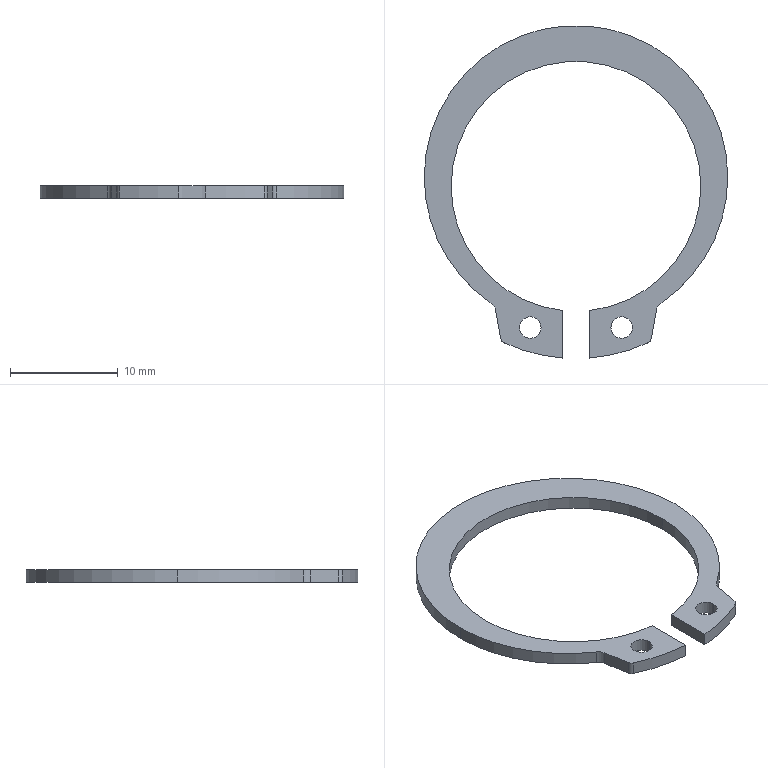Part | SolidWorks | features Extrusion 1 | 1 solid | 22 faces | box 28.2 x 30.881 x 1.2 mm | volume 270.422 mm3 | cylinder 16 | plane 6 | commonest cylinder face diameters 2 x6 23.2 x3 28.2 x3 1 x2 32 x2
STEP:
#1=CARTESIAN_POINT('',(-3.25,-13.959,0.));
#2=VERTEX_POINT('',#1);
#3=CARTESIAN_POINT('',(-5.25,-13.959,0.));
#4=VERTEX_POINT('',#3);
#5=CARTESIAN_POINT('',(-4.25,-13.959,0.));
#6=DIRECTION('',(0.,0.,-1.));
#7=DIRECTION('',(1.,0.,0.));
#8=AXIS2_PLACEMENT_3D('',#5,#6,#7);
#9=CIRCLE('',#8,1.);
#10=EDGE_CURVE('',#2,#4,#9,.T.);
#11=ORIENTED_EDGE('',*,*,#10,.F.);
#12=CARTESIAN_POINT('',(-3.25,-13.959,-1.2));
#13=VERTEX_POINT('',#12);
#14=CARTESIAN_POINT('',(-3.25,-13.959,0.));
#15=DIRECTION('',(0.,0.,-1.));
#16=VECTOR('',#15,1000.);
#17=LINE('',#14,#16);
#18=EDGE_CURVE('',#2,#13,#17,.T.);
#19=ORIENTED_EDGE('',*,*,#18,.T.);
#20=CARTESIAN_POINT('',(-5.25,-13.959,-1.2));
#21=VERTEX_POINT('',#20);
#22=CARTESIAN_POINT('',(-4.25,-13.959,-1.2));
#23=DIRECTION('',(0.,0.,-1.));
#24=DIRECTION('',(1.,0.,0.));
#25=AXIS2_PLACEMENT_3D('',#22,#23,#24);
#26=CIRCLE('',#25,1.);
#27=EDGE_CURVE('',#13,#21,#26,.T.);
#28=ORIENTED_EDGE('',*,*,#27,.T.);
#29=CARTESIAN_POINT('',(-5.25,-13.959,0.));
#30=DIRECTION('',(0.,0.,-1.));
#31=VECTOR('',#30,1000.);
#32=LINE('',#29,#31);
#33=EDGE_CURVE('',#4,#21,#32,.T.);
#34=ORIENTED_EDGE('',*,*,#33,.F.);
#35=EDGE_LOOP('',(#11,#19,#28,#34));
#36=FACE_OUTER_BOUND('',#35,.T.);
#37=CARTESIAN_POINT('',(-4.25,-13.959,0.));
#38=DIRECTION('',(0.,0.,-1.));
#39=DIRECTION('',(-1.,0.,0.));
#40=AXIS2_PLACEMENT_3D('',#37,#38,#39);
#41=CYLINDRICAL_SURFACE('',#40,1.);
#42=ADVANCED_FACE('',(#36),#41,.F.);
#43=CARTESIAN_POINT('',(5.25,-13.959,0.));
#44=VERTEX_POINT('',#43);
#45=CARTESIAN_POINT('',(3.25,-13.959,0.));
#46=VERTEX_POINT('',#45);
#47=CARTESIAN_POINT('',(4.25,-13.959,0.));
#48=DIRECTION('',(0.,0.,-1.));
#49=DIRECTION('',(1.,0.,0.));
#50=AXIS2_PLACEMENT_3D('',#47,#48,#49);
#51=CIRCLE('',#50,1.);
#52=EDGE_CURVE('',#44,#46,#51,.T.);
#53=ORIENTED_EDGE('',*,*,#52,.F.);
#54=CARTESIAN_POINT('',(5.25,-13.959,-1.2));
#55=VERTEX_POINT('',#54);
#56=CARTESIAN_POINT('',(5.25,-13.959,0.));
#57=DIRECTION('',(0.,0.,-1.));
#58=VECTOR('',#57,1000.);
#59=LINE('',#56,#58);
#60=EDGE_CURVE('',#44,#55,#59,.T.);
#61=ORIENTED_EDGE('',*,*,#60,.T.);
#62=CARTESIAN_POINT('',(3.25,-13.959,-1.2));
#63=VERTEX_POINT('',#62);
#64=CARTESIAN_POINT('',(4.25,-13.959,-1.2));
#65=DIRECTION('',(0.,0.,-1.));
#66=DIRECTION('',(1.,0.,0.));
#67=AXIS2_PLACEMENT_3D('',#64,#65,#66);
#68=CIRCLE('',#67,1.);
#69=EDGE_CURVE('',#55,#63,#68,.T.);
#70=ORIENTED_EDGE('',*,*,#69,.T.);
#71=CARTESIAN_POINT('',(3.25,-13.959,0.));
#72=DIRECTION('',(0.,0.,-1.));
#73=VECTOR('',#72,1000.);
#74=LINE('',#71,#73);
#75=EDGE_CURVE('',#46,#63,#74,.T.);
#76=ORIENTED_EDGE('',*,*,#75,.F.);
#77=EDGE_LOOP('',(#53,#61,#70,#76));
#78=FACE_OUTER_BOUND('',#77,.T.);
#79=CARTESIAN_POINT('',(4.25,-13.959,0.));
#80=DIRECTION('',(0.,0.,-1.));
#81=DIRECTION('',(-1.,0.,0.));
#82=AXIS2_PLACEMENT_3D('',#79,#80,#81);
#83=CYLINDRICAL_SURFACE('',#82,1.);
#84=ADVANCED_FACE('',(#78),#83,.F.);
#85=CARTESIAN_POINT('',(1.25,-12.362,0.));
#86=VERTEX_POINT('',#85);
#87=CARTESIAN_POINT('',(11.6,-0.83,0.));
#88=VERTEX_POINT('',#87);
#89=CARTESIAN_POINT('',(0.,-0.83,0.));
#90=DIRECTION('',(0.,0.,1.));
#91=DIRECTION('',(1.,0.,0.));
#92=AXIS2_PLACEMENT_3D('',#89,#90,#91);
#93=CIRCLE('',#92,11.6);
#94=EDGE_CURVE('',#86,#88,#93,.T.);
#95=ORIENTED_EDGE('',*,*,#94,.T.);
#96=CARTESIAN_POINT('',(11.6,-0.83,-1.2));
#97=VERTEX_POINT('',#96);
#98=CARTESIAN_POINT('',(11.6,-0.83,0.));
#99=DIRECTION('',(0.,0.,-1.));
#100=VECTOR('',#99,1000.);
#101=LINE('',#98,#100);
#102=EDGE_CURVE('',#88,#97,#101,.T.);
#103=ORIENTED_EDGE('',*,*,#102,.T.);
#104=CARTESIAN_POINT('',(1.25,-12.362,-1.2));
#105=VERTEX_POINT('',#104);
#106=CARTESIAN_POINT('',(0.,-0.83,-1.2));
#107=DIRECTION('',(0.,0.,1.));
#108=DIRECTION('',(1.,0.,0.));
#109=AXIS2_PLACEMENT_3D('',#106,#107,#108);
#110=CIRCLE('',#109,11.6);
#111=EDGE_CURVE('',#105,#97,#110,.T.);
#112=ORIENTED_EDGE('',*,*,#111,.F.);
#113=CARTESIAN_POINT('',(1.25,-12.362,0.));
#114=DIRECTION('',(0.,0.,-1.));
#115=VECTOR('',#114,1000.);
#116=LINE('',#113,#115);
#117=EDGE_CURVE('',#86,#105,#116,.T.);
#118=ORIENTED_EDGE('',*,*,#117,.F.);
#119=EDGE_LOOP('',(#95,#103,#112,#118));
#120=FACE_OUTER_BOUND('',#119,.T.);
#121=CARTESIAN_POINT('',(0.,-0.83,0.));
#122=DIRECTION('',(0.,0.,-1.));
#123=DIRECTION('',(-1.,0.,0.));
#124=AXIS2_PLACEMENT_3D('',#121,#122,#123);
#125=CYLINDRICAL_SURFACE('',#124,11.6);
#126=ADVANCED_FACE('',(#120),#125,.F.);
#127=ORIENTED_EDGE('',*,*,#102,.F.);
#128=CARTESIAN_POINT('',(-11.6,-0.83,0.));
#129=VERTEX_POINT('',#128);
#130=CARTESIAN_POINT('',(0.,-0.83,0.));
#131=DIRECTION('',(0.,0.,1.));
#132=DIRECTION('',(1.,0.,0.));
#133=AXIS2_PLACEMENT_3D('',#130,#131,#132);
#134=CIRCLE('',#133,11.6);
#135=EDGE_CURVE('',#88,#129,#134,.T.);
#136=ORIENTED_EDGE('',*,*,#135,.T.);
#137=CARTESIAN_POINT('',(-11.6,-0.83,-1.2));
#138=VERTEX_POINT('',#137);
#139=CARTESIAN_POINT('',(-11.6,-0.83,0.));
#140=DIRECTION('',(0.,0.,-1.));
#141=VECTOR('',#140,1000.);
#142=LINE('',#139,#141);
#143=EDGE_CURVE('',#129,#138,#142,.T.);
#144=ORIENTED_EDGE('',*,*,#143,.T.);
#145=CARTESIAN_POINT('',(0.,-0.83,-1.2));
#146=DIRECTION('',(0.,0.,1.));
#147=DIRECTION('',(1.,0.,0.));
#148=AXIS2_PLACEMENT_3D('',#145,#146,#147);
#149=CIRCLE('',#148,11.6);
#150=EDGE_CURVE('',#97,#138,#149,.T.);
#151=ORIENTED_EDGE('',*,*,#150,.F.);
#152=EDGE_LOOP('',(#127,#136,#144,#151));
#153=FACE_OUTER_BOUND('',#152,.T.);
#154=CARTESIAN_POINT('',(0.,-0.83,0.));
#155=DIRECTION('',(0.,0.,-1.));
#156=DIRECTION('',(-1.,0.,0.));
#157=AXIS2_PLACEMENT_3D('',#154,#155,#156);
#158=CYLINDRICAL_SURFACE('',#157,11.6);
#159=ADVANCED_FACE('',(#153),#158,.F.);
#160=CARTESIAN_POINT('',(-14.1,0.,0.));
#161=VERTEX_POINT('',#160);
#162=CARTESIAN_POINT('',(14.1,0.,0.));
#163=VERTEX_POINT('',#162);
#164=CARTESIAN_POINT('',(0.,0.,0.));
#165=DIRECTION('',(0.,0.,-1.));
#166=DIRECTION('',(-1.,0.,0.));
#167=AXIS2_PLACEMENT_3D('',#164,#165,#166);
#168=CIRCLE('',#167,14.1);
#169=EDGE_CURVE('',#161,#163,#168,.T.);
#170=ORIENTED_EDGE('',*,*,#169,.T.);
#171=CARTESIAN_POINT('',(14.1,0.,-1.2));
#172=VERTEX_POINT('',#171);
#173=CARTESIAN_POINT('',(14.1,0.,0.));
#174=DIRECTION('',(0.,0.,-1.));
#175=VECTOR('',#174,1000.);
#176=LINE('',#173,#175);
#177=EDGE_CURVE('',#163,#172,#176,.T.);
#178=ORIENTED_EDGE('',*,*,#177,.T.);
#179=CARTESIAN_POINT('',(-14.1,0.,-1.2));
#180=VERTEX_POINT('',#179);
#181=CARTESIAN_POINT('',(0.,0.,-1.2));
#182=DIRECTION('',(0.,0.,-1.));
#183=DIRECTION('',(-1.,0.,0.));
#184=AXIS2_PLACEMENT_3D('',#181,#182,#183);
#185=CIRCLE('',#184,14.1);
#186=EDGE_CURVE('',#180,#172,#185,.T.);
#187=ORIENTED_EDGE('',*,*,#186,.F.);
#188=CARTESIAN_POINT('',(-14.1,0.,0.));
#189=DIRECTION('',(0.,0.,-1.));
#190=VECTOR('',#189,1000.);
#191=LINE('',#188,#190);
#192=EDGE_CURVE('',#161,#180,#191,.T.);
#193=ORIENTED_EDGE('',*,*,#192,.F.);
#194=EDGE_LOOP('',(#170,#178,#187,#193));
#195=FACE_OUTER_BOUND('',#194,.T.);
#196=CARTESIAN_POINT('',(0.,0.,0.));
#197=DIRECTION('',(0.,0.,-1.));
#198=DIRECTION('',(-1.,0.,0.));
#199=AXIS2_PLACEMENT_3D('',#196,#197,#198);
#200=CYLINDRICAL_SURFACE('',#199,14.1);
#201=ADVANCED_FACE('',(#195),#200,.T.);
#202=CARTESIAN_POINT('',(-7.893,-11.684,0.));
#203=VERTEX_POINT('',#202);
#204=CARTESIAN_POINT('',(0.,0.,0.));
#205=DIRECTION('',(0.,0.,-1.));
#206=DIRECTION('',(-1.,0.,0.));
#207=AXIS2_PLACEMENT_3D('',#204,#205,#206);
#208=CIRCLE('',#207,14.1);
#209=EDGE_CURVE('',#203,#161,#208,.T.);
#210=ORIENTED_EDGE('',*,*,#209,.T.);
#211=ORIENTED_EDGE('',*,*,#192,.T.);
#212=CARTESIAN_POINT('',(-7.893,-11.684,-1.2));
#213=VERTEX_POINT('',#212);
#214=CARTESIAN_POINT('',(0.,0.,-1.2));
#215=DIRECTION('',(0.,0.,-1.));
#216=DIRECTION('',(-1.,0.,0.));
#217=AXIS2_PLACEMENT_3D('',#214,#215,#216);
#218=CIRCLE('',#217,14.1);
#219=EDGE_CURVE('',#213,#180,#218,.T.);
#220=ORIENTED_EDGE('',*,*,#219,.F.);
#221=CARTESIAN_POINT('',(-7.893,-11.684,0.));
#222=DIRECTION('',(0.,0.,-1.));
#223=VECTOR('',#222,1000.);
#224=LINE('',#221,#223);
#225=EDGE_CURVE('',#203,#213,#224,.T.);
#226=ORIENTED_EDGE('',*,*,#225,.F.);
#227=EDGE_LOOP('',(#210,#211,#220,#226));
#228=FACE_OUTER_BOUND('',#227,.T.);
#229=CARTESIAN_POINT('',(0.,0.,0.));
#230=DIRECTION('',(0.,0.,-1.));
#231=DIRECTION('',(-1.,0.,0.));
#232=AXIS2_PLACEMENT_3D('',#229,#230,#231);
#233=CYLINDRICAL_SURFACE('',#232,14.1);
#234=ADVANCED_FACE('',(#228),#233,.T.);
#235=CARTESIAN_POINT('',(6.719,-15.351,-1.2));
#236=VERTEX_POINT('',#235);
#237=CARTESIAN_POINT('',(1.25,-16.781,-1.2));
#238=VERTEX_POINT('',#237);
#239=CARTESIAN_POINT('',(0.,-0.83,-1.2));
#240=DIRECTION('',(0.,0.,-1.));
#241=DIRECTION('',(-1.,0.,0.));
#242=AXIS2_PLACEMENT_3D('',#239,#240,#241);
#243=CIRCLE('',#242,16.);
#244=EDGE_CURVE('',#236,#238,#243,.T.);
#245=ORIENTED_EDGE('',*,*,#244,.F.);
#246=CARTESIAN_POINT('',(6.719,-15.351,0.));
#247=VERTEX_POINT('',#246);
#248=CARTESIAN_POINT('',(6.719,-15.351,0.));
#249=DIRECTION('',(0.,0.,-1.));
#250=VECTOR('',#249,1000.);
#251=LINE('',#248,#250);
#252=EDGE_CURVE('',#247,#236,#251,.T.);
#253=ORIENTED_EDGE('',*,*,#252,.F.);
#254=CARTESIAN_POINT('',(1.25,-16.781,0.));
#255=VERTEX_POINT('',#254);
#256=CARTESIAN_POINT('',(0.,-0.83,0.));
#257=DIRECTION('',(0.,0.,-1.));
#258=DIRECTION('',(-1.,0.,0.));
#259=AXIS2_PLACEMENT_3D('',#256,#257,#258);
#260=CIRCLE('',#259,16.);
#261=EDGE_CURVE('',#247,#255,#260,.T.);
#262=ORIENTED_EDGE('',*,*,#261,.T.);
#263=CARTESIAN_POINT('',(1.25,-16.781,0.));
#264=DIRECTION('',(0.,0.,-1.));
#265=VECTOR('',#264,1000.);
#266=LINE('',#263,#265);
#267=EDGE_CURVE('',#255,#238,#266,.T.);
#268=ORIENTED_EDGE('',*,*,#267,.T.);
#269=EDGE_LOOP('',(#245,#253,#262,#268));
#270=FACE_OUTER_BOUND('',#269,.T.);
#271=CARTESIAN_POINT('',(0.,-0.83,0.));
#272=DIRECTION('',(0.,0.,-1.));
#273=DIRECTION('',(-1.,0.,0.));
#274=AXIS2_PLACEMENT_3D('',#271,#272,#273);
#275=CYLINDRICAL_SURFACE('',#274,16.);
#276=ADVANCED_FACE('',(#270),#275,.T.);
#277=CARTESIAN_POINT('',(7.002,-14.984,-1.2));
#278=VERTEX_POINT('',#277);
#279=CARTESIAN_POINT('',(6.509,-14.897,-1.2));
#280=DIRECTION('',(0.,0.,-1.));
#281=DIRECTION('',(-1.,0.,0.));
#282=AXIS2_PLACEMENT_3D('',#279,#280,#281);
#283=CIRCLE('',#282,0.5);
#284=EDGE_CURVE('',#278,#236,#283,.T.);
#285=ORIENTED_EDGE('',*,*,#284,.F.);
#286=CARTESIAN_POINT('',(7.002,-14.984,0.));
#287=VERTEX_POINT('',#286);
#288=CARTESIAN_POINT('',(7.002,-14.984,0.));
#289=DIRECTION('',(0.,0.,-1.));
#290=VECTOR('',#289,1000.);
#291=LINE('',#288,#290);
#292=EDGE_CURVE('',#287,#278,#291,.T.);
#293=ORIENTED_EDGE('',*,*,#292,.F.);
#294=CARTESIAN_POINT('',(6.509,-14.897,0.));
#295=DIRECTION('',(0.,0.,-1.));
#296=DIRECTION('',(-1.,0.,0.));
#297=AXIS2_PLACEMENT_3D('',#294,#295,#296);
#298=CIRCLE('',#297,0.5);
#299=EDGE_CURVE('',#287,#247,#298,.T.);
#300=ORIENTED_EDGE('',*,*,#299,.T.);
#301=ORIENTED_EDGE('',*,*,#252,.T.);
#302=EDGE_LOOP('',(#285,#293,#300,#301));
#303=FACE_OUTER_BOUND('',#302,.T.);
#304=CARTESIAN_POINT('',(6.509,-14.897,0.));
#305=DIRECTION('',(0.,0.,-1.));
#306=DIRECTION('',(-1.,0.,0.));
#307=AXIS2_PLACEMENT_3D('',#304,#305,#306);
#308=CYLINDRICAL_SURFACE('',#307,0.5);
#309=ADVANCED_FACE('',(#303),#308,.T.);
#310=CARTESIAN_POINT('',(7.468,-12.339,-1.2));
#311=VERTEX_POINT('',#310);
#312=CARTESIAN_POINT('',(7.468,-12.339,-1.2));
#313=DIRECTION('',(-0.1736,-0.9848,0.));
#314=VECTOR('',#313,1000.);
#315=LINE('',#312,#314);
#316=EDGE_CURVE('',#311,#278,#315,.T.);
#317=ORIENTED_EDGE('',*,*,#316,.F.);
#318=CARTESIAN_POINT('',(7.468,-12.339,0.));
#319=VERTEX_POINT('',#318);
#320=CARTESIAN_POINT('',(7.468,-12.339,0.));
#321=DIRECTION('',(0.,0.,-1.));
#322=VECTOR('',#321,1000.);
#323=LINE('',#320,#322);
#324=EDGE_CURVE('',#319,#311,#323,.T.);
#325=ORIENTED_EDGE('',*,*,#324,.F.);
#326=CARTESIAN_POINT('',(7.468,-12.339,0.));
#327=DIRECTION('',(-0.1736,-0.9848,0.));
#328=VECTOR('',#327,1000.);
#329=LINE('',#326,#328);
#330=EDGE_CURVE('',#319,#287,#329,.T.);
#331=ORIENTED_EDGE('',*,*,#330,.T.);
#332=ORIENTED_EDGE('',*,*,#292,.T.);
#333=EDGE_LOOP('',(#317,#325,#331,#332));
#334=FACE_OUTER_BOUND('',#333,.T.);
#335=CARTESIAN_POINT('',(7.468,-12.339,0.));
#336=DIRECTION('',(0.9848,-0.1736,0.));
#337=DIRECTION('',(0.1736,0.9848,0.));
#338=AXIS2_PLACEMENT_3D('',#335,#336,#337);
#339=PLANE('',#338);
#340=ADVANCED_FACE('',(#334),#339,.T.);
#341=CARTESIAN_POINT('',(7.893,-11.684,-1.2));
#342=VERTEX_POINT('',#341);
#343=CARTESIAN_POINT('',(8.453,-12.512,-1.2));
#344=DIRECTION('',(0.,0.,1.));
#345=DIRECTION('',(1.,0.,0.));
#346=AXIS2_PLACEMENT_3D('',#343,#344,#345);
#347=CIRCLE('',#346,1.);
#348=EDGE_CURVE('',#342,#311,#347,.T.);
#349=ORIENTED_EDGE('',*,*,#348,.F.);
#350=CARTESIAN_POINT('',(7.893,-11.684,0.));
#351=VERTEX_POINT('',#350);
#352=CARTESIAN_POINT('',(7.893,-11.684,0.));
#353=DIRECTION('',(0.,0.,-1.));
#354=VECTOR('',#353,1000.);
#355=LINE('',#352,#354);
#356=EDGE_CURVE('',#351,#342,#355,.T.);
#357=ORIENTED_EDGE('',*,*,#356,.F.);
#358=CARTESIAN_POINT('',(8.453,-12.512,0.));
#359=DIRECTION('',(0.,0.,1.));
#360=DIRECTION('',(1.,0.,0.));
#361=AXIS2_PLACEMENT_3D('',#358,#359,#360);
#362=CIRCLE('',#361,1.);
#363=EDGE_CURVE('',#351,#319,#362,.T.);
#364=ORIENTED_EDGE('',*,*,#363,.T.);
#365=ORIENTED_EDGE('',*,*,#324,.T.);
#366=EDGE_LOOP('',(#349,#357,#364,#365));
#367=FACE_OUTER_BOUND('',#366,.T.);
#368=CARTESIAN_POINT('',(8.453,-12.512,0.));
#369=DIRECTION('',(0.,0.,-1.));
#370=DIRECTION('',(-1.,0.,0.));
#371=AXIS2_PLACEMENT_3D('',#368,#369,#370);
#372=CYLINDRICAL_SURFACE('',#371,1.);
#373=ADVANCED_FACE('',(#367),#372,.F.);
#374=ORIENTED_EDGE('',*,*,#177,.F.);
#375=CARTESIAN_POINT('',(0.,0.,0.));
#376=DIRECTION('',(0.,0.,-1.));
#377=DIRECTION('',(-1.,0.,0.));
#378=AXIS2_PLACEMENT_3D('',#375,#376,#377);
#379=CIRCLE('',#378,14.1);
#380=EDGE_CURVE('',#163,#351,#379,.T.);
#381=ORIENTED_EDGE('',*,*,#380,.T.);
#382=ORIENTED_EDGE('',*,*,#356,.T.);
#383=CARTESIAN_POINT('',(0.,0.,-1.2));
#384=DIRECTION('',(0.,0.,-1.));
#385=DIRECTION('',(-1.,0.,0.));
#386=AXIS2_PLACEMENT_3D('',#383,#384,#385);
#387=CIRCLE('',#386,14.1);
#388=EDGE_CURVE('',#172,#342,#387,.T.);
#389=ORIENTED_EDGE('',*,*,#388,.F.);
#390=EDGE_LOOP('',(#374,#381,#382,#389));
#391=FACE_OUTER_BOUND('',#390,.T.);
#392=CARTESIAN_POINT('',(0.,0.,0.));
#393=DIRECTION('',(0.,0.,-1.));
#394=DIRECTION('',(-1.,0.,0.));
#395=AXIS2_PLACEMENT_3D('',#392,#393,#394);
#396=CYLINDRICAL_SURFACE('',#395,14.1);
#397=ADVANCED_FACE('',(#391),#396,.T.);
#398=CARTESIAN_POINT('',(-7.468,-12.339,-1.2));
#399=VERTEX_POINT('',#398);
#400=CARTESIAN_POINT('',(-8.453,-12.512,-1.2));
#401=DIRECTION('',(0.,0.,1.));
#402=DIRECTION('',(1.,0.,0.));
#403=AXIS2_PLACEMENT_3D('',#400,#401,#402);
#404=CIRCLE('',#403,1.);
#405=EDGE_CURVE('',#399,#213,#404,.T.);
#406=ORIENTED_EDGE('',*,*,#405,.F.);
#407=CARTESIAN_POINT('',(-7.468,-12.339,0.));
#408=VERTEX_POINT('',#407);
#409=CARTESIAN_POINT('',(-7.468,-12.339,0.));
#410=DIRECTION('',(0.,0.,-1.));
#411=VECTOR('',#410,1000.);
#412=LINE('',#409,#411);
#413=EDGE_CURVE('',#408,#399,#412,.T.);
#414=ORIENTED_EDGE('',*,*,#413,.F.);
#415=CARTESIAN_POINT('',(-8.453,-12.512,0.));
#416=DIRECTION('',(0.,0.,1.));
#417=DIRECTION('',(1.,0.,0.));
#418=AXIS2_PLACEMENT_3D('',#415,#416,#417);
#419=CIRCLE('',#418,1.);
#420=EDGE_CURVE('',#408,#203,#419,.T.);
#421=ORIENTED_EDGE('',*,*,#420,.T.);
#422=ORIENTED_EDGE('',*,*,#225,.T.);
#423=EDGE_LOOP('',(#406,#414,#421,#422));
#424=FACE_OUTER_BOUND('',#423,.T.);
#425=CARTESIAN_POINT('',(-8.453,-12.512,0.));
#426=DIRECTION('',(0.,0.,-1.));
#427=DIRECTION('',(-1.,0.,0.));
#428=AXIS2_PLACEMENT_3D('',#425,#426,#427);
#429=CYLINDRICAL_SURFACE('',#428,1.);
#430=ADVANCED_FACE('',(#424),#429,.F.);
#431=CARTESIAN_POINT('',(-7.002,-14.984,-1.2));
#432=VERTEX_POINT('',#431);
#433=CARTESIAN_POINT('',(-7.002,-14.984,-1.2));
#434=DIRECTION('',(-0.1736,0.9848,0.));
#435=VECTOR('',#434,1000.);
#436=LINE('',#433,#435);
#437=EDGE_CURVE('',#432,#399,#436,.T.);
#438=ORIENTED_EDGE('',*,*,#437,.F.);
#439=CARTESIAN_POINT('',(-7.002,-14.984,0.));
#440=VERTEX_POINT('',#439);
#441=CARTESIAN_POINT('',(-7.002,-14.984,0.));
#442=DIRECTION('',(0.,0.,-1.));
#443=VECTOR('',#442,1000.);
#444=LINE('',#441,#443);
#445=EDGE_CURVE('',#440,#432,#444,.T.);
#446=ORIENTED_EDGE('',*,*,#445,.F.);
#447=CARTESIAN_POINT('',(-7.002,-14.984,0.));
#448=DIRECTION('',(-0.1736,0.9848,0.));
#449=VECTOR('',#448,1000.);
#450=LINE('',#447,#449);
#451=EDGE_CURVE('',#440,#408,#450,.T.);
#452=ORIENTED_EDGE('',*,*,#451,.T.);
#453=ORIENTED_EDGE('',*,*,#413,.T.);
#454=EDGE_LOOP('',(#438,#446,#452,#453));
#455=FACE_OUTER_BOUND('',#454,.T.);
#456=CARTESIAN_POINT('',(-7.002,-14.984,0.));
#457=DIRECTION('',(-0.9848,-0.1736,0.));
#458=DIRECTION('',(0.1736,-0.9848,0.));
#459=AXIS2_PLACEMENT_3D('',#456,#457,#458);
#460=PLANE('',#459);
#461=ADVANCED_FACE('',(#455),#460,.T.);
#462=CARTESIAN_POINT('',(-6.719,-15.351,-1.2));
#463=VERTEX_POINT('',#462);
#464=CARTESIAN_POINT('',(-6.509,-14.897,-1.2));
#465=DIRECTION('',(0.,0.,-1.));
#466=DIRECTION('',(-1.,0.,0.));
#467=AXIS2_PLACEMENT_3D('',#464,#465,#466);
#468=CIRCLE('',#467,0.5);
#469=EDGE_CURVE('',#463,#432,#468,.T.);
#470=ORIENTED_EDGE('',*,*,#469,.F.);
#471=CARTESIAN_POINT('',(-6.719,-15.351,0.));
#472=VERTEX_POINT('',#471);
#473=CARTESIAN_POINT('',(-6.719,-15.351,0.));
#474=DIRECTION('',(0.,0.,-1.));
#475=VECTOR('',#474,1000.);
#476=LINE('',#473,#475);
#477=EDGE_CURVE('',#472,#463,#476,.T.);
#478=ORIENTED_EDGE('',*,*,#477,.F.);
#479=CARTESIAN_POINT('',(-6.509,-14.897,0.));
#480=DIRECTION('',(0.,0.,-1.));
#481=DIRECTION('',(-1.,0.,0.));
#482=AXIS2_PLACEMENT_3D('',#479,#480,#481);
#483=CIRCLE('',#482,0.5);
#484=EDGE_CURVE('',#472,#440,#483,.T.);
#485=ORIENTED_EDGE('',*,*,#484,.T.);
#486=ORIENTED_EDGE('',*,*,#445,.T.);
#487=EDGE_LOOP('',(#470,#478,#485,#486));
#488=FACE_OUTER_BOUND('',#487,.T.);
#489=CARTESIAN_POINT('',(-6.509,-14.897,0.));
#490=DIRECTION('',(0.,0.,-1.));
#491=DIRECTION('',(-1.,0.,0.));
#492=AXIS2_PLACEMENT_3D('',#489,#490,#491);
#493=CYLINDRICAL_SURFACE('',#492,0.5);
#494=ADVANCED_FACE('',(#488),#493,.T.);
#495=CARTESIAN_POINT('',(-1.25,-16.781,-1.2));
#496=VERTEX_POINT('',#495);
#497=CARTESIAN_POINT('',(0.,-0.83,-1.2));
#498=DIRECTION('',(0.,0.,-1.));
#499=DIRECTION('',(-1.,0.,0.));
#500=AXIS2_PLACEMENT_3D('',#497,#498,#499);
#501=CIRCLE('',#500,16.);
#502=EDGE_CURVE('',#496,#463,#501,.T.);
#503=ORIENTED_EDGE('',*,*,#502,.F.);
#504=CARTESIAN_POINT('',(-1.25,-16.781,0.));
#505=VERTEX_POINT('',#504);
#506=CARTESIAN_POINT('',(-1.25,-16.781,0.));
#507=DIRECTION('',(0.,0.,-1.));
#508=VECTOR('',#507,1000.);
#509=LINE('',#506,#508);
#510=EDGE_CURVE('',#505,#496,#509,.T.);
#511=ORIENTED_EDGE('',*,*,#510,.F.);
#512=CARTESIAN_POINT('',(0.,-0.83,0.));
#513=DIRECTION('',(0.,0.,-1.));
#514=DIRECTION('',(-1.,0.,0.));
#515=AXIS2_PLACEMENT_3D('',#512,#513,#514);
#516=CIRCLE('',#515,16.);
#517=EDGE_CURVE('',#505,#472,#516,.T.);
#518=ORIENTED_EDGE('',*,*,#517,.T.);
#519=ORIENTED_EDGE('',*,*,#477,.T.);
#520=EDGE_LOOP('',(#503,#511,#518,#519));
#521=FACE_OUTER_BOUND('',#520,.T.);
#522=CARTESIAN_POINT('',(0.,-0.83,0.));
#523=DIRECTION('',(0.,0.,-1.));
#524=DIRECTION('',(-1.,0.,0.));
#525=AXIS2_PLACEMENT_3D('',#522,#523,#524);
#526=CYLINDRICAL_SURFACE('',#525,16.);
#527=ADVANCED_FACE('',(#521),#526,.T.);
#528=CARTESIAN_POINT('',(-1.25,-12.362,-1.2));
#529=VERTEX_POINT('',#528);
#530=CARTESIAN_POINT('',(-1.25,-12.362,-1.2));
#531=DIRECTION('',(0.,-1.,0.));
#532=VECTOR('',#531,1000.);
#533=LINE('',#530,#532);
#534=EDGE_CURVE('',#529,#496,#533,.T.);
#535=ORIENTED_EDGE('',*,*,#534,.F.);
#536=CARTESIAN_POINT('',(-1.25,-12.362,0.));
#537=VERTEX_POINT('',#536);
#538=CARTESIAN_POINT('',(-1.25,-12.362,0.));
#539=DIRECTION('',(0.,0.,-1.));
#540=VECTOR('',#539,1000.);
#541=LINE('',#538,#540);
#542=EDGE_CURVE('',#537,#529,#541,.T.);
#543=ORIENTED_EDGE('',*,*,#542,.F.);
#544=CARTESIAN_POINT('',(-1.25,-12.362,0.));
#545=DIRECTION('',(0.,-1.,0.));
#546=VECTOR('',#545,1000.);
#547=LINE('',#544,#546);
#548=EDGE_CURVE('',#537,#505,#547,.T.);
#549=ORIENTED_EDGE('',*,*,#548,.T.);
#550=ORIENTED_EDGE('',*,*,#510,.T.);
#551=EDGE_LOOP('',(#535,#543,#549,#550));
#552=FACE_OUTER_BOUND('',#551,.T.);
#553=CARTESIAN_POINT('',(-1.25,-12.362,0.));
#554=DIRECTION('',(1.,0.,0.));
#555=DIRECTION('',(0.,0.,-1.));
#556=AXIS2_PLACEMENT_3D('',#553,#554,#555);
#557=PLANE('',#556);
#558=ADVANCED_FACE('',(#552),#557,.T.);
#559=ORIENTED_EDGE('',*,*,#143,.F.);
#560=CARTESIAN_POINT('',(0.,-0.83,0.));
#561=DIRECTION('',(0.,0.,1.));
#562=DIRECTION('',(1.,0.,0.));
#563=AXIS2_PLACEMENT_3D('',#560,#561,#562);
#564=CIRCLE('',#563,11.6);
#565=EDGE_CURVE('',#129,#537,#564,.T.);
#566=ORIENTED_EDGE('',*,*,#565,.T.);
#567=ORIENTED_EDGE('',*,*,#542,.T.);
#568=CARTESIAN_POINT('',(0.,-0.83,-1.2));
#569=DIRECTION('',(0.,0.,1.));
#570=DIRECTION('',(1.,0.,0.));
#571=AXIS2_PLACEMENT_3D('',#568,#569,#570);
#572=CIRCLE('',#571,11.6);
#573=EDGE_CURVE('',#138,#529,#572,.T.);
#574=ORIENTED_EDGE('',*,*,#573,.F.);
#575=EDGE_LOOP('',(#559,#566,#567,#574));
#576=FACE_OUTER_BOUND('',#575,.T.);
#577=CARTESIAN_POINT('',(0.,-0.83,0.));
#578=DIRECTION('',(0.,0.,-1.));
#579=DIRECTION('',(-1.,0.,0.));
#580=AXIS2_PLACEMENT_3D('',#577,#578,#579);
#581=CYLINDRICAL_SURFACE('',#580,11.6);
#582=ADVANCED_FACE('',(#576),#581,.F.);
#583=CARTESIAN_POINT('',(1.25,-16.781,-1.2));
#584=DIRECTION('',(0.,1.,0.));
#585=VECTOR('',#584,1000.);
#586=LINE('',#583,#585);
#587=EDGE_CURVE('',#238,#105,#586,.T.);
#588=ORIENTED_EDGE('',*,*,#587,.F.);
#589=ORIENTED_EDGE('',*,*,#267,.F.);
#590=CARTESIAN_POINT('',(1.25,-16.781,0.));
#591=DIRECTION('',(0.,1.,0.));
#592=VECTOR('',#591,1000.);
#593=LINE('',#590,#592);
#594=EDGE_CURVE('',#255,#86,#593,.T.);
#595=ORIENTED_EDGE('',*,*,#594,.T.);
#596=ORIENTED_EDGE('',*,*,#117,.T.);
#597=EDGE_LOOP('',(#588,#589,#595,#596));
#598=FACE_OUTER_BOUND('',#597,.T.);
#599=CARTESIAN_POINT('',(1.25,-16.781,0.));
#600=DIRECTION('',(-1.,0.,0.));
#601=DIRECTION('',(0.,0.,1.));
#602=AXIS2_PLACEMENT_3D('',#599,#600,#601);
#603=PLANE('',#602);
#604=ADVANCED_FACE('',(#598),#603,.T.);
#605=CARTESIAN_POINT('',(-4.25,-13.959,0.));
#606=DIRECTION('',(0.,0.,-1.));
#607=DIRECTION('',(1.,0.,0.));
#608=AXIS2_PLACEMENT_3D('',#605,#606,#607);
#609=CIRCLE('',#608,1.);
#610=EDGE_CURVE('',#4,#2,#609,.T.);
#611=ORIENTED_EDGE('',*,*,#610,.T.);
#612=ORIENTED_EDGE('',*,*,#10,.T.);
#613=EDGE_LOOP('',(#611,#612));
#614=FACE_BOUND('',#613,.T.);
#615=CARTESIAN_POINT('',(4.25,-13.959,0.));
#616=DIRECTION('',(0.,0.,-1.));
#617=DIRECTION('',(1.,0.,0.));
#618=AXIS2_PLACEMENT_3D('',#615,#616,#617);
#619=CIRCLE('',#618,1.);
#620=EDGE_CURVE('',#46,#44,#619,.T.);
#621=ORIENTED_EDGE('',*,*,#620,.T.);
#622=ORIENTED_EDGE('',*,*,#52,.T.);
#623=EDGE_LOOP('',(#621,#622));
#624=FACE_BOUND('',#623,.T.);
#625=ORIENTED_EDGE('',*,*,#261,.F.);
#626=ORIENTED_EDGE('',*,*,#299,.F.);
#627=ORIENTED_EDGE('',*,*,#330,.F.);
#628=ORIENTED_EDGE('',*,*,#363,.F.);
#629=ORIENTED_EDGE('',*,*,#380,.F.);
#630=ORIENTED_EDGE('',*,*,#169,.F.);
#631=ORIENTED_EDGE('',*,*,#209,.F.);
#632=ORIENTED_EDGE('',*,*,#420,.F.);
#633=ORIENTED_EDGE('',*,*,#451,.F.);
#634=ORIENTED_EDGE('',*,*,#484,.F.);
#635=ORIENTED_EDGE('',*,*,#517,.F.);
#636=ORIENTED_EDGE('',*,*,#548,.F.);
#637=ORIENTED_EDGE('',*,*,#565,.F.);
#638=ORIENTED_EDGE('',*,*,#135,.F.);
#639=ORIENTED_EDGE('',*,*,#94,.F.);
#640=ORIENTED_EDGE('',*,*,#594,.F.);
#641=EDGE_LOOP('',(#625,#626,#627,#628,#629,#630,#631,#632,#633,#634,#635,#636,#637,#638,#639,#640));
#642=FACE_OUTER_BOUND('',#641,.T.);
#643=CARTESIAN_POINT('',(0.,-0.83,0.));
#644=DIRECTION('',(0.,0.,-1.));
#645=DIRECTION('',(-1.,0.,0.));
#646=AXIS2_PLACEMENT_3D('',#643,#644,#645);
#647=PLANE('',#646);
#648=ADVANCED_FACE('',(#614,#624,#642),#647,.F.);
#649=CARTESIAN_POINT('',(-4.25,-13.959,-1.2));
#650=DIRECTION('',(0.,0.,-1.));
#651=DIRECTION('',(1.,0.,0.));
#652=AXIS2_PLACEMENT_3D('',#649,#650,#651);
#653=CIRCLE('',#652,1.);
#654=EDGE_CURVE('',#21,#13,#653,.T.);
#655=ORIENTED_EDGE('',*,*,#654,.F.);
#656=ORIENTED_EDGE('',*,*,#27,.F.);
#657=EDGE_LOOP('',(#655,#656));
#658=FACE_BOUND('',#657,.T.);
#659=CARTESIAN_POINT('',(4.25,-13.959,-1.2));
#660=DIRECTION('',(0.,0.,-1.));
#661=DIRECTION('',(1.,0.,0.));
#662=AXIS2_PLACEMENT_3D('',#659,#660,#661);
#663=CIRCLE('',#662,1.);
#664=EDGE_CURVE('',#63,#55,#663,.T.);
#665=ORIENTED_EDGE('',*,*,#664,.F.);
#666=ORIENTED_EDGE('',*,*,#69,.F.);
#667=EDGE_LOOP('',(#665,#666));
#668=FACE_BOUND('',#667,.T.);
#669=ORIENTED_EDGE('',*,*,#244,.T.);
#670=ORIENTED_EDGE('',*,*,#587,.T.);
#671=ORIENTED_EDGE('',*,*,#111,.T.);
#672=ORIENTED_EDGE('',*,*,#150,.T.);
#673=ORIENTED_EDGE('',*,*,#573,.T.);
#674=ORIENTED_EDGE('',*,*,#534,.T.);
#675=ORIENTED_EDGE('',*,*,#502,.T.);
#676=ORIENTED_EDGE('',*,*,#469,.T.);
#677=ORIENTED_EDGE('',*,*,#437,.T.);
#678=ORIENTED_EDGE('',*,*,#405,.T.);
#679=ORIENTED_EDGE('',*,*,#219,.T.);
#680=ORIENTED_EDGE('',*,*,#186,.T.);
#681=ORIENTED_EDGE('',*,*,#388,.T.);
#682=ORIENTED_EDGE('',*,*,#348,.T.);
#683=ORIENTED_EDGE('',*,*,#316,.T.);
#684=ORIENTED_EDGE('',*,*,#284,.T.);
#685=EDGE_LOOP('',(#669,#670,#671,#672,#673,#674,#675,#676,#677,#678,#679,#680,#681,#682,#683,#684));
#686=FACE_OUTER_BOUND('',#685,.T.);
#687=CARTESIAN_POINT('',(0.,-0.83,-1.2));
#688=DIRECTION('',(0.,0.,-1.));
#689=DIRECTION('',(-1.,0.,0.));
#690=AXIS2_PLACEMENT_3D('',#687,#688,#689);
#691=PLANE('',#690);
#692=ADVANCED_FACE('',(#658,#668,#686),#691,.T.);
#693=ORIENTED_EDGE('',*,*,#60,.F.);
#694=ORIENTED_EDGE('',*,*,#620,.F.);
#695=ORIENTED_EDGE('',*,*,#75,.T.);
#696=ORIENTED_EDGE('',*,*,#664,.T.);
#697=EDGE_LOOP('',(#693,#694,#695,#696));
#698=FACE_OUTER_BOUND('',#697,.T.);
#699=CARTESIAN_POINT('',(4.25,-13.959,0.));
#700=DIRECTION('',(0.,0.,-1.));
#701=DIRECTION('',(-1.,0.,0.));
#702=AXIS2_PLACEMENT_3D('',#699,#700,#701);
#703=CYLINDRICAL_SURFACE('',#702,1.);
#704=ADVANCED_FACE('',(#698),#703,.F.);
#705=ORIENTED_EDGE('',*,*,#18,.F.);
#706=ORIENTED_EDGE('',*,*,#610,.F.);
#707=ORIENTED_EDGE('',*,*,#33,.T.);
#708=ORIENTED_EDGE('',*,*,#654,.T.);
#709=EDGE_LOOP('',(#705,#706,#707,#708));
#710=FACE_OUTER_BOUND('',#709,.T.);
#711=CARTESIAN_POINT('',(-4.25,-13.959,0.));
#712=DIRECTION('',(0.,0.,-1.));
#713=DIRECTION('',(-1.,0.,0.));
#714=AXIS2_PLACEMENT_3D('',#711,#712,#713);
#715=CYLINDRICAL_SURFACE('',#714,1.);
#716=ADVANCED_FACE('',(#710),#715,.F.);
#717=CLOSED_SHELL('',(#42,#84,#126,#159,#201,#234,#276,#309,#340,#373,#397,#430,#461,#494,#527,#558,#582,#604,#648,#692,#704,#716));
#718=MANIFOLD_SOLID_BREP('',#717);
#719=CARTESIAN_POINT('',(0.,0.,0.));
#720=DIRECTION('',(0.,0.,1.));
#721=DIRECTION('',(1.,0.,0.));
#722=AXIS2_PLACEMENT_3D('',#719,#720,#721);
#723=(LENGTH_UNIT()NAMED_UNIT(*)SI_UNIT(.MILLI.,.METRE.));
#724=UNCERTAINTY_MEASURE_WITH_UNIT(LENGTH_MEASURE(0.00001),#723,'','');
#725=(NAMED_UNIT(*)PLANE_ANGLE_UNIT()SI_UNIT($,.RADIAN.));
#726=(NAMED_UNIT(*)SI_UNIT($,.STERADIAN.)SOLID_ANGLE_UNIT());
#727=(GEOMETRIC_REPRESENTATION_CONTEXT(3)GLOBAL_UNCERTAINTY_ASSIGNED_CONTEXT((#724))GLOBAL_UNIT_ASSIGNED_CONTEXT((#723,#725,#726))REPRESENTATION_CONTEXT('',''));
#728=ADVANCED_BREP_SHAPE_REPRESENTATION('',(#718,#722),#727);